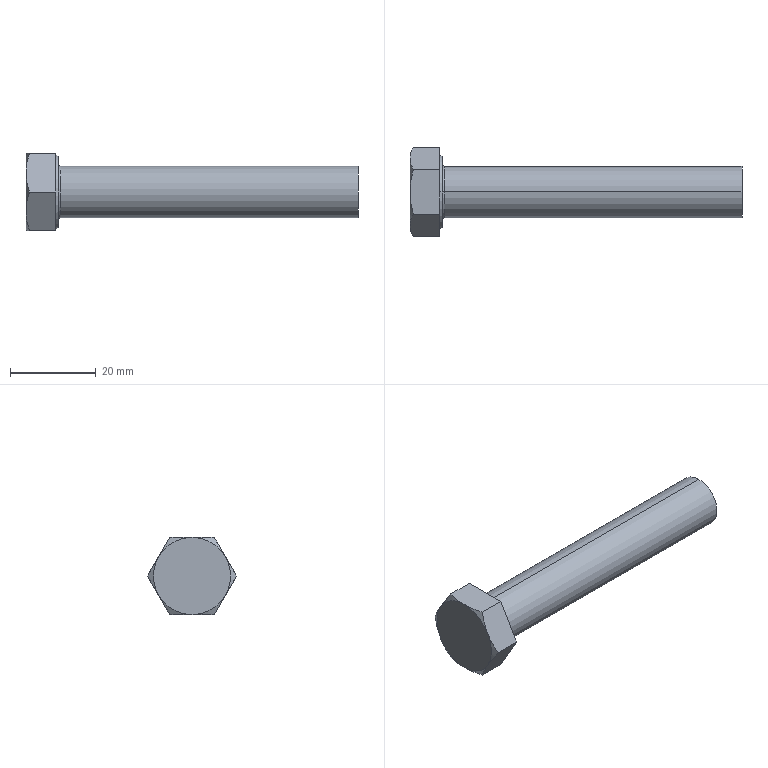Part | SolidWorks | features RevCut 3, Extrusion 1, Fillet 1, LPattern 1, Revolution 1 | 1 solid | 22 faces | box 77.5 x 20.785 x 18 mm | volume 9985 mm3 | plane 10 | cone 8 | torus 2 | cylinder 2 | commonest cylinder face diameters 12 x2
STEP:
#1=CARTESIAN_POINT('',(8.1,0.,6.));
#2=VERTEX_POINT('',#1);
#3=CARTESIAN_POINT('',(8.1,0.,-6.));
#4=VERTEX_POINT('',#3);
#5=CARTESIAN_POINT('',(8.1,0.,0.));
#6=DIRECTION('',(1.,0.,0.));
#7=DIRECTION('',(0.,0.,-1.));
#8=AXIS2_PLACEMENT_3D('',#5,#6,#7);
#9=CIRCLE('',#8,6.);
#10=EDGE_CURVE('',#2,#4,#9,.T.);
#11=ORIENTED_EDGE('',*,*,#10,.F.);
#12=CARTESIAN_POINT('',(7.5,0.,6.6));
#13=VERTEX_POINT('',#12);
#14=CARTESIAN_POINT('',(8.1,0.,6.6));
#15=DIRECTION('',(0.,1.,0.));
#16=DIRECTION('',(0.,0.,1.));
#17=AXIS2_PLACEMENT_3D('',#14,#15,#16);
#18=CIRCLE('',#17,0.6);
#19=EDGE_CURVE('',#2,#13,#18,.T.);
#20=ORIENTED_EDGE('',*,*,#19,.T.);
#21=CARTESIAN_POINT('',(7.5,0.,-6.6));
#22=VERTEX_POINT('',#21);
#23=CARTESIAN_POINT('',(7.5,0.,0.));
#24=DIRECTION('',(-1.,0.,0.));
#25=DIRECTION('',(0.,0.,-1.));
#26=AXIS2_PLACEMENT_3D('',#23,#24,#25);
#27=CIRCLE('',#26,6.6);
#28=EDGE_CURVE('',#22,#13,#27,.T.);
#29=ORIENTED_EDGE('',*,*,#28,.F.);
#30=CARTESIAN_POINT('',(8.1,0.,-6.6));
#31=DIRECTION('',(0.,-1.,0.));
#32=DIRECTION('',(0.,0.,-1.));
#33=AXIS2_PLACEMENT_3D('',#30,#31,#32);
#34=CIRCLE('',#33,0.6);
#35=EDGE_CURVE('',#4,#22,#34,.T.);
#36=ORIENTED_EDGE('',*,*,#35,.F.);
#37=EDGE_LOOP('',(#11,#20,#29,#36));
#38=FACE_OUTER_BOUND('',#37,.T.);
#39=CARTESIAN_POINT('',(8.1,0.,0.));
#40=DIRECTION('',(1.,0.,0.));
#41=DIRECTION('',(0.,0.,-1.));
#42=AXIS2_PLACEMENT_3D('',#39,#40,#41);
#43=TOROIDAL_SURFACE('',#42,6.6,0.6);
#44=ADVANCED_FACE('',(#38),#43,.F.);
#45=CARTESIAN_POINT('',(77.5,0.,6.));
#46=VERTEX_POINT('',#45);
#47=CARTESIAN_POINT('',(77.5,0.,-6.));
#48=VERTEX_POINT('',#47);
#49=CARTESIAN_POINT('',(77.5,0.,0.));
#50=DIRECTION('',(-1.,0.,0.));
#51=DIRECTION('',(0.,0.,1.));
#52=AXIS2_PLACEMENT_3D('',#49,#50,#51);
#53=CIRCLE('',#52,6.);
#54=EDGE_CURVE('',#46,#48,#53,.T.);
#55=ORIENTED_EDGE('',*,*,#54,.T.);
#56=CARTESIAN_POINT('',(0.,0.,-6.));
#57=DIRECTION('',(-1.,0.,0.));
#58=VECTOR('',#57,1000.);
#59=LINE('',#56,#58);
#60=EDGE_CURVE('',#48,#4,#59,.T.);
#61=ORIENTED_EDGE('',*,*,#60,.T.);
#62=CARTESIAN_POINT('',(8.1,0.,0.));
#63=DIRECTION('',(1.,0.,0.));
#64=DIRECTION('',(0.,0.,-1.));
#65=AXIS2_PLACEMENT_3D('',#62,#63,#64);
#66=CIRCLE('',#65,6.);
#67=EDGE_CURVE('',#4,#2,#66,.T.);
#68=ORIENTED_EDGE('',*,*,#67,.T.);
#69=CARTESIAN_POINT('',(0.,0.,6.));
#70=DIRECTION('',(-1.,0.,0.));
#71=VECTOR('',#70,1000.);
#72=LINE('',#69,#71);
#73=EDGE_CURVE('',#46,#2,#72,.T.);
#74=ORIENTED_EDGE('',*,*,#73,.F.);
#75=EDGE_LOOP('',(#55,#61,#68,#74));
#76=FACE_OUTER_BOUND('',#75,.T.);
#77=CARTESIAN_POINT('',(0.,0.,0.));
#78=DIRECTION('',(-1.,0.,0.));
#79=DIRECTION('',(0.,0.,1.));
#80=AXIS2_PLACEMENT_3D('',#77,#78,#79);
#81=CYLINDRICAL_SURFACE('',#80,6.);
#82=ADVANCED_FACE('',(#76),#81,.T.);
#83=CARTESIAN_POINT('',(7.5,0.,8.315));
#84=VERTEX_POINT('',#83);
#85=CARTESIAN_POINT('',(7.5,0.,-8.315));
#86=VERTEX_POINT('',#85);
#87=CARTESIAN_POINT('',(7.5,0.,0.));
#88=DIRECTION('',(-1.,0.,0.));
#89=DIRECTION('',(0.,0.,1.));
#90=AXIS2_PLACEMENT_3D('',#87,#88,#89);
#91=CIRCLE('',#90,8.315);
#92=EDGE_CURVE('',#84,#86,#91,.T.);
#93=ORIENTED_EDGE('',*,*,#92,.T.);
#94=CARTESIAN_POINT('',(6.9,0.,-8.661));
#95=VERTEX_POINT('',#94);
#96=CARTESIAN_POINT('',(6.9,0.,-8.661));
#97=DIRECTION('',(-0.866,0.,-0.5));
#98=VECTOR('',#97,1000.);
#99=LINE('',#96,#98);
#100=EDGE_CURVE('',#86,#95,#99,.T.);
#101=ORIENTED_EDGE('',*,*,#100,.T.);
#102=CARTESIAN_POINT('',(6.9,0.,8.661));
#103=VERTEX_POINT('',#102);
#104=CARTESIAN_POINT('',(6.9,0.,0.));
#105=DIRECTION('',(-1.,0.,0.));
#106=DIRECTION('',(0.,0.,1.));
#107=AXIS2_PLACEMENT_3D('',#104,#105,#106);
#108=CIRCLE('',#107,8.661);
#109=EDGE_CURVE('',#103,#95,#108,.T.);
#110=ORIENTED_EDGE('',*,*,#109,.F.);
#111=CARTESIAN_POINT('',(6.9,0.,8.661));
#112=DIRECTION('',(-0.866,0.,0.5));
#113=VECTOR('',#112,1000.);
#114=LINE('',#111,#113);
#115=EDGE_CURVE('',#84,#103,#114,.T.);
#116=ORIENTED_EDGE('',*,*,#115,.F.);
#117=EDGE_LOOP('',(#93,#101,#110,#116));
#118=FACE_OUTER_BOUND('',#117,.T.);
#119=CARTESIAN_POINT('',(6.9,0.,0.));
#120=DIRECTION('',(-1.,0.,0.));
#121=DIRECTION('',(0.,0.,1.));
#122=AXIS2_PLACEMENT_3D('',#119,#120,#121);
#123=CONICAL_SURFACE('',#122,8.661,0.5236);
#124=ADVANCED_FACE('',(#118),#123,.T.);
#125=CARTESIAN_POINT('',(6.9,5.196,-9.));
#126=VERTEX_POINT('',#125);
#127=CARTESIAN_POINT('',(6.9,10.392,0.));
#128=VERTEX_POINT('',#127);
#129=CARTESIAN_POINT('',(6.9,5.196,-9.));
#130=DIRECTION('',(0.,0.5,0.866));
#131=VECTOR('',#130,1000.);
#132=LINE('',#129,#131);
#133=EDGE_CURVE('',#126,#128,#132,.T.);
#134=ORIENTED_EDGE('',*,*,#133,.F.);
#135=CARTESIAN_POINT('',(0.8038,5.196,-9.));
#136=VERTEX_POINT('',#135);
#137=CARTESIAN_POINT('',(7.5,5.196,-9.));
#138=DIRECTION('',(-1.,0.,0.));
#139=VECTOR('',#138,1000.);
#140=LINE('',#137,#139);
#141=EDGE_CURVE('',#126,#136,#140,.T.);
#142=ORIENTED_EDGE('',*,*,#141,.T.);
#143=CARTESIAN_POINT('',(0.,7.794,-4.5));
#144=VERTEX_POINT('',#143);
#145=CARTESIAN_POINT('',(0.,7.794,-4.5));
#146=CARTESIAN_POINT('',(0.,7.574,-4.882));
#147=CARTESIAN_POINT('',(0.019,7.352,-5.266));
#148=CARTESIAN_POINT('',(0.09253,6.914,-6.024));
#149=CARTESIAN_POINT('',(0.147,6.697,-6.401));
#150=CARTESIAN_POINT('',(0.357,6.048,-7.525));
#151=CARTESIAN_POINT('',(0.5591,5.62,-8.266));
#152=CARTESIAN_POINT('',(0.8038,5.196,-9.));
#153=B_SPLINE_CURVE_WITH_KNOTS('',3,(#145,#146,#147,#148,#149,#150,#151,#152),.UNSPECIFIED.,.F.,.F.,(4,2,2,4),(0.005258,0.006567,0.007877,0.0105),.UNSPECIFIED.);
#154=EDGE_CURVE('',#144,#136,#153,.T.);
#155=ORIENTED_EDGE('',*,*,#154,.F.);
#156=CARTESIAN_POINT('',(0.8038,10.392,0.));
#157=VERTEX_POINT('',#156);
#158=CARTESIAN_POINT('',(0.8038,10.392,0.));
#159=CARTESIAN_POINT('',(0.5585,9.967,-0.7361));
#160=CARTESIAN_POINT('',(0.3563,9.539,-1.478));
#161=CARTESIAN_POINT('',(0.07661,8.674,-2.976));
#162=CARTESIAN_POINT('',(0.,8.237,-3.733));
#163=CARTESIAN_POINT('',(0.,7.794,-4.5));
#164=B_SPLINE_CURVE_WITH_KNOTS('',3,(#158,#159,#160,#161,#162,#163),.UNSPECIFIED.,.F.,.F.,(4,2,4),(0.000000238,0.002629,0.005258),.UNSPECIFIED.);
#165=EDGE_CURVE('',#157,#144,#164,.T.);
#166=ORIENTED_EDGE('',*,*,#165,.F.);
#167=CARTESIAN_POINT('',(7.5,10.392,0.));
#168=DIRECTION('',(-1.,0.,0.));
#169=VECTOR('',#168,1000.);
#170=LINE('',#167,#169);
#171=EDGE_CURVE('',#128,#157,#170,.T.);
#172=ORIENTED_EDGE('',*,*,#171,.F.);
#173=EDGE_LOOP('',(#134,#142,#155,#166,#172));
#174=FACE_OUTER_BOUND('',#173,.T.);
#175=CARTESIAN_POINT('',(7.5,5.196,-9.));
#176=DIRECTION('',(0.,-0.866,0.5));
#177=DIRECTION('',(0.,-0.5,-0.866));
#178=AXIS2_PLACEMENT_3D('',#175,#176,#177);
#179=PLANE('',#178);
#180=ADVANCED_FACE('',(#174),#179,.F.);
#181=CARTESIAN_POINT('',(6.9,5.196,9.));
#182=VERTEX_POINT('',#181);
#183=CARTESIAN_POINT('',(6.9,10.392,0.));
#184=DIRECTION('',(0.,-0.5,0.866));
#185=VECTOR('',#184,1000.);
#186=LINE('',#183,#185);
#187=EDGE_CURVE('',#128,#182,#186,.T.);
#188=ORIENTED_EDGE('',*,*,#187,.F.);
#189=ORIENTED_EDGE('',*,*,#171,.T.);
#190=CARTESIAN_POINT('',(0.,7.794,4.5));
#191=VERTEX_POINT('',#190);
#192=CARTESIAN_POINT('',(0.,7.794,4.5));
#193=CARTESIAN_POINT('',(0.,8.015,4.118));
#194=CARTESIAN_POINT('',(0.019,8.236,3.734));
#195=CARTESIAN_POINT('',(0.09253,8.674,2.976));
#196=CARTESIAN_POINT('',(0.147,8.892,2.599));
#197=CARTESIAN_POINT('',(0.357,9.541,1.475));
#198=CARTESIAN_POINT('',(0.5591,9.968,0.7343));
#199=CARTESIAN_POINT('',(0.8038,10.392,0.));
#200=B_SPLINE_CURVE_WITH_KNOTS('',3,(#192,#193,#194,#195,#196,#197,#198,#199),.UNSPECIFIED.,.F.,.F.,(4,2,2,4),(0.005258,0.006567,0.007877,0.0105),.UNSPECIFIED.);
#201=EDGE_CURVE('',#191,#157,#200,.T.);
#202=ORIENTED_EDGE('',*,*,#201,.F.);
#203=CARTESIAN_POINT('',(0.8038,5.196,9.));
#204=VERTEX_POINT('',#203);
#205=CARTESIAN_POINT('',(0.8038,5.196,9.));
#206=CARTESIAN_POINT('',(0.5585,5.621,8.264));
#207=CARTESIAN_POINT('',(0.3563,6.049,7.522));
#208=CARTESIAN_POINT('',(0.07661,6.914,6.024));
#209=CARTESIAN_POINT('',(0.,7.352,5.267));
#210=CARTESIAN_POINT('',(0.,7.794,4.5));
#211=B_SPLINE_CURVE_WITH_KNOTS('',3,(#205,#206,#207,#208,#209,#210),.UNSPECIFIED.,.F.,.F.,(4,2,4),(0.000000238,0.002629,0.005258),.UNSPECIFIED.);
#212=EDGE_CURVE('',#204,#191,#211,.T.);
#213=ORIENTED_EDGE('',*,*,#212,.F.);
#214=CARTESIAN_POINT('',(7.5,5.196,9.));
#215=DIRECTION('',(-1.,0.,0.));
#216=VECTOR('',#215,1000.);
#217=LINE('',#214,#216);
#218=EDGE_CURVE('',#182,#204,#217,.T.);
#219=ORIENTED_EDGE('',*,*,#218,.F.);
#220=EDGE_LOOP('',(#188,#189,#202,#213,#219));
#221=FACE_OUTER_BOUND('',#220,.T.);
#222=CARTESIAN_POINT('',(7.5,10.392,0.));
#223=DIRECTION('',(0.,-0.866,-0.5));
#224=DIRECTION('',(0.,0.5,-0.866));
#225=AXIS2_PLACEMENT_3D('',#222,#223,#224);
#226=PLANE('',#225);
#227=ADVANCED_FACE('',(#221),#226,.F.);
#228=CARTESIAN_POINT('',(6.9,-5.196,9.));
#229=VERTEX_POINT('',#228);
#230=CARTESIAN_POINT('',(6.9,5.196,9.));
#231=DIRECTION('',(0.,-1.,0.));
#232=VECTOR('',#231,1000.);
#233=LINE('',#230,#232);
#234=EDGE_CURVE('',#182,#229,#233,.T.);
#235=ORIENTED_EDGE('',*,*,#234,.F.);
#236=ORIENTED_EDGE('',*,*,#218,.T.);
#237=CARTESIAN_POINT('',(0.,0.,9.));
#238=VERTEX_POINT('',#237);
#239=CARTESIAN_POINT('',(0.,0.,9.));
#240=CARTESIAN_POINT('',(0.,0.4401,9.));
#241=CARTESIAN_POINT('',(0.01885,0.8832,9.));
#242=CARTESIAN_POINT('',(0.09319,1.767,9.));
#243=CARTESIAN_POINT('',(0.1482,2.204,9.));
#244=CARTESIAN_POINT('',(0.3593,3.505,9.));
#245=CARTESIAN_POINT('',(0.5612,4.356,9.));
#246=CARTESIAN_POINT('',(0.8038,5.196,9.));
#247=B_SPLINE_CURVE_WITH_KNOTS('',3,(#239,#240,#241,#242,#243,#244,#245,#246),.UNSPECIFIED.,.F.,.F.,(4,2,2,4),(0.01498,0.0163,0.01761,0.02025),.UNSPECIFIED.);
#248=EDGE_CURVE('',#238,#204,#247,.T.);
#249=ORIENTED_EDGE('',*,*,#248,.F.);
#250=CARTESIAN_POINT('',(0.8038,-5.196,9.));
#251=VERTEX_POINT('',#250);
#252=CARTESIAN_POINT('',(0.8038,-5.196,9.));
#253=CARTESIAN_POINT('',(0.5595,-4.35,9.));
#254=CARTESIAN_POINT('',(0.3552,-3.485,9.));
#255=CARTESIAN_POINT('',(0.07569,-1.752,9.));
#256=CARTESIAN_POINT('',(0.,-0.8794,9.));
#257=CARTESIAN_POINT('',(0.,0.,9.));
#258=B_SPLINE_CURVE_WITH_KNOTS('',3,(#252,#253,#254,#255,#256,#257),.UNSPECIFIED.,.F.,.F.,(4,2,4),(0.00972,0.01235,0.01498),.UNSPECIFIED.);
#259=EDGE_CURVE('',#251,#238,#258,.T.);
#260=ORIENTED_EDGE('',*,*,#259,.F.);
#261=CARTESIAN_POINT('',(7.5,-5.196,9.));
#262=DIRECTION('',(-1.,0.,0.));
#263=VECTOR('',#262,1000.);
#264=LINE('',#261,#263);
#265=EDGE_CURVE('',#229,#251,#264,.T.);
#266=ORIENTED_EDGE('',*,*,#265,.F.);
#267=EDGE_LOOP('',(#235,#236,#249,#260,#266));
#268=FACE_OUTER_BOUND('',#267,.T.);
#269=CARTESIAN_POINT('',(7.5,5.196,9.));
#270=DIRECTION('',(0.,0.,-1.));
#271=DIRECTION('',(-1.,0.,0.));
#272=AXIS2_PLACEMENT_3D('',#269,#270,#271);
#273=PLANE('',#272);
#274=ADVANCED_FACE('',(#268),#273,.F.);
#275=CARTESIAN_POINT('',(6.9,-10.392,0.));
#276=VERTEX_POINT('',#275);
#277=CARTESIAN_POINT('',(6.9,-10.392,0.));
#278=DIRECTION('',(0.,-0.5,-0.866));
#279=VECTOR('',#278,1000.);
#280=LINE('',#277,#279);
#281=EDGE_CURVE('',#229,#276,#280,.T.);
#282=ORIENTED_EDGE('',*,*,#281,.F.);
#283=ORIENTED_EDGE('',*,*,#265,.T.);
#284=CARTESIAN_POINT('',(0.,-7.794,4.5));
#285=VERTEX_POINT('',#284);
#286=CARTESIAN_POINT('',(0.,-7.794,4.5));
#287=CARTESIAN_POINT('',(0.,-7.574,4.882));
#288=CARTESIAN_POINT('',(0.019,-7.352,5.266));
#289=CARTESIAN_POINT('',(0.09253,-6.914,6.024));
#290=CARTESIAN_POINT('',(0.147,-6.697,6.401));
#291=CARTESIAN_POINT('',(0.357,-6.048,7.525));
#292=CARTESIAN_POINT('',(0.5591,-5.62,8.266));
#293=CARTESIAN_POINT('',(0.8038,-5.196,9.));
#294=B_SPLINE_CURVE_WITH_KNOTS('',3,(#286,#287,#288,#289,#290,#291,#292,#293),.UNSPECIFIED.,.F.,.F.,(4,2,2,4),(0.005258,0.006567,0.007877,0.0105),.UNSPECIFIED.);
#295=EDGE_CURVE('',#285,#251,#294,.T.);
#296=ORIENTED_EDGE('',*,*,#295,.F.);
#297=CARTESIAN_POINT('',(0.8038,-10.392,0.));
#298=VERTEX_POINT('',#297);
#299=CARTESIAN_POINT('',(0.8038,-10.392,0.));
#300=CARTESIAN_POINT('',(0.5585,-9.967,0.7361));
#301=CARTESIAN_POINT('',(0.3563,-9.539,1.478));
#302=CARTESIAN_POINT('',(0.07661,-8.674,2.976));
#303=CARTESIAN_POINT('',(0.,-8.237,3.733));
#304=CARTESIAN_POINT('',(0.,-7.794,4.5));
#305=B_SPLINE_CURVE_WITH_KNOTS('',3,(#299,#300,#301,#302,#303,#304),.UNSPECIFIED.,.F.,.F.,(4,2,4),(0.000000238,0.002629,0.005258),.UNSPECIFIED.);
#306=EDGE_CURVE('',#298,#285,#305,.T.);
#307=ORIENTED_EDGE('',*,*,#306,.F.);
#308=CARTESIAN_POINT('',(7.5,-10.392,0.));
#309=DIRECTION('',(-1.,0.,0.));
#310=VECTOR('',#309,1000.);
#311=LINE('',#308,#310);
#312=EDGE_CURVE('',#276,#298,#311,.T.);
#313=ORIENTED_EDGE('',*,*,#312,.F.);
#314=EDGE_LOOP('',(#282,#283,#296,#307,#313));
#315=FACE_OUTER_BOUND('',#314,.T.);
#316=CARTESIAN_POINT('',(7.5,-10.392,0.));
#317=DIRECTION('',(0.,0.866,-0.5));
#318=DIRECTION('',(0.,0.5,0.866));
#319=AXIS2_PLACEMENT_3D('',#316,#317,#318);
#320=PLANE('',#319);
#321=ADVANCED_FACE('',(#315),#320,.F.);
#322=CARTESIAN_POINT('',(6.9,-5.196,-9.));
#323=VERTEX_POINT('',#322);
#324=CARTESIAN_POINT('',(6.9,-5.196,-9.));
#325=DIRECTION('',(0.,0.5,-0.866));
#326=VECTOR('',#325,1000.);
#327=LINE('',#324,#326);
#328=EDGE_CURVE('',#276,#323,#327,.T.);
#329=ORIENTED_EDGE('',*,*,#328,.F.);
#330=ORIENTED_EDGE('',*,*,#312,.T.);
#331=CARTESIAN_POINT('',(0.,-7.794,-4.5));
#332=VERTEX_POINT('',#331);
#333=CARTESIAN_POINT('',(0.,-7.794,-4.5));
#334=CARTESIAN_POINT('',(0.,-8.015,-4.118));
#335=CARTESIAN_POINT('',(0.019,-8.236,-3.734));
#336=CARTESIAN_POINT('',(0.09253,-8.674,-2.976));
#337=CARTESIAN_POINT('',(0.147,-8.892,-2.599));
#338=CARTESIAN_POINT('',(0.357,-9.541,-1.475));
#339=CARTESIAN_POINT('',(0.5591,-9.968,-0.7343));
#340=CARTESIAN_POINT('',(0.8038,-10.392,0.));
#341=B_SPLINE_CURVE_WITH_KNOTS('',3,(#333,#334,#335,#336,#337,#338,#339,#340),.UNSPECIFIED.,.F.,.F.,(4,2,2,4),(0.005258,0.006567,0.007877,0.0105),.UNSPECIFIED.);
#342=EDGE_CURVE('',#332,#298,#341,.T.);
#343=ORIENTED_EDGE('',*,*,#342,.F.);
#344=CARTESIAN_POINT('',(0.8038,-5.196,-9.));
#345=VERTEX_POINT('',#344);
#346=CARTESIAN_POINT('',(0.8038,-5.196,-9.));
#347=CARTESIAN_POINT('',(0.5585,-5.621,-8.264));
#348=CARTESIAN_POINT('',(0.3563,-6.049,-7.522));
#349=CARTESIAN_POINT('',(0.07661,-6.914,-6.024));
#350=CARTESIAN_POINT('',(0.,-7.352,-5.267));
#351=CARTESIAN_POINT('',(0.,-7.794,-4.5));
#352=B_SPLINE_CURVE_WITH_KNOTS('',3,(#346,#347,#348,#349,#350,#351),.UNSPECIFIED.,.F.,.F.,(4,2,4),(0.000000238,0.002629,0.005258),.UNSPECIFIED.);
#353=EDGE_CURVE('',#345,#332,#352,.T.);
#354=ORIENTED_EDGE('',*,*,#353,.F.);
#355=CARTESIAN_POINT('',(7.5,-5.196,-9.));
#356=DIRECTION('',(-1.,0.,0.));
#357=VECTOR('',#356,1000.);
#358=LINE('',#355,#357);
#359=EDGE_CURVE('',#323,#345,#358,.T.);
#360=ORIENTED_EDGE('',*,*,#359,.F.);
#361=EDGE_LOOP('',(#329,#330,#343,#354,#360));
#362=FACE_OUTER_BOUND('',#361,.T.);
#363=CARTESIAN_POINT('',(7.5,-5.196,-9.));
#364=DIRECTION('',(0.,0.866,0.5));
#365=DIRECTION('',(0.,-0.5,0.866));
#366=AXIS2_PLACEMENT_3D('',#363,#364,#365);
#367=PLANE('',#366);
#368=ADVANCED_FACE('',(#362),#367,.F.);
#369=CARTESIAN_POINT('',(6.9,5.196,-9.));
#370=DIRECTION('',(0.,1.,0.));
#371=VECTOR('',#370,1000.);
#372=LINE('',#369,#371);
#373=EDGE_CURVE('',#323,#126,#372,.T.);
#374=ORIENTED_EDGE('',*,*,#373,.F.);
#375=ORIENTED_EDGE('',*,*,#359,.T.);
#376=CARTESIAN_POINT('',(0.,0.,-9.));
#377=VERTEX_POINT('',#376);
#378=CARTESIAN_POINT('',(0.,0.,-9.));
#379=CARTESIAN_POINT('',(0.,-0.8794,-9.));
#380=CARTESIAN_POINT('',(0.07569,-1.752,-9.));
#381=CARTESIAN_POINT('',(0.3552,-3.485,-9.));
#382=CARTESIAN_POINT('',(0.5595,-4.35,-9.));
#383=CARTESIAN_POINT('',(0.8038,-5.196,-9.));
#384=B_SPLINE_CURVE_WITH_KNOTS('',3,(#378,#379,#380,#381,#382,#383),.UNSPECIFIED.,.F.,.F.,(4,2,4),(0.03045,0.03308,0.03571),.UNSPECIFIED.);
#385=EDGE_CURVE('',#377,#345,#384,.T.);
#386=ORIENTED_EDGE('',*,*,#385,.F.);
#387=CARTESIAN_POINT('',(0.8038,5.196,-9.));
#388=CARTESIAN_POINT('',(0.5612,4.356,-9.));
#389=CARTESIAN_POINT('',(0.3593,3.505,-9.));
#390=CARTESIAN_POINT('',(0.1482,2.204,-9.));
#391=CARTESIAN_POINT('',(0.09319,1.767,-9.));
#392=CARTESIAN_POINT('',(0.01885,0.8832,-9.));
#393=CARTESIAN_POINT('',(0.,0.4401,-9.));
#394=CARTESIAN_POINT('',(0.,0.,-9.));
#395=B_SPLINE_CURVE_WITH_KNOTS('',3,(#387,#388,#389,#390,#391,#392,#393,#394),.UNSPECIFIED.,.F.,.F.,(4,2,2,4),(0.02519,0.02782,0.02914,0.03045),.UNSPECIFIED.);
#396=EDGE_CURVE('',#136,#377,#395,.T.);
#397=ORIENTED_EDGE('',*,*,#396,.F.);
#398=ORIENTED_EDGE('',*,*,#141,.F.);
#399=EDGE_LOOP('',(#374,#375,#386,#397,#398));
#400=FACE_OUTER_BOUND('',#399,.T.);
#401=CARTESIAN_POINT('',(7.5,5.196,-9.));
#402=DIRECTION('',(0.,0.,1.));
#403=DIRECTION('',(0.,-1.,0.));
#404=AXIS2_PLACEMENT_3D('',#401,#402,#403);
#405=PLANE('',#404);
#406=ADVANCED_FACE('',(#400),#405,.F.);
#407=ORIENTED_EDGE('',*,*,#353,.T.);
#408=CARTESIAN_POINT('',(0.,0.,0.));
#409=DIRECTION('',(1.,0.,0.));
#410=DIRECTION('',(0.,0.,-1.));
#411=AXIS2_PLACEMENT_3D('',#408,#409,#410);
#412=CIRCLE('',#411,9.);
#413=EDGE_CURVE('',#332,#377,#412,.T.);
#414=ORIENTED_EDGE('',*,*,#413,.T.);
#415=ORIENTED_EDGE('',*,*,#385,.T.);
#416=EDGE_LOOP('',(#407,#414,#415));
#417=FACE_OUTER_BOUND('',#416,.T.);
#418=CARTESIAN_POINT('',(0.,0.,0.));
#419=DIRECTION('',(1.,0.,0.));
#420=DIRECTION('',(0.,0.,-1.));
#421=AXIS2_PLACEMENT_3D('',#418,#419,#420);
#422=CONICAL_SURFACE('',#421,9.,1.047);
#423=ADVANCED_FACE('',(#417),#422,.T.);
#424=ORIENTED_EDGE('',*,*,#306,.T.);
#425=CARTESIAN_POINT('',(0.,0.,0.));
#426=DIRECTION('',(1.,0.,0.));
#427=DIRECTION('',(0.,0.,-1.));
#428=AXIS2_PLACEMENT_3D('',#425,#426,#427);
#429=CIRCLE('',#428,9.);
#430=EDGE_CURVE('',#285,#332,#429,.T.);
#431=ORIENTED_EDGE('',*,*,#430,.T.);
#432=ORIENTED_EDGE('',*,*,#342,.T.);
#433=EDGE_LOOP('',(#424,#431,#432));
#434=FACE_OUTER_BOUND('',#433,.T.);
#435=CARTESIAN_POINT('',(0.,0.,0.));
#436=DIRECTION('',(1.,0.,0.));
#437=DIRECTION('',(0.,0.,-1.));
#438=AXIS2_PLACEMENT_3D('',#435,#436,#437);
#439=CONICAL_SURFACE('',#438,9.,1.047);
#440=ADVANCED_FACE('',(#434),#439,.T.);
#441=ORIENTED_EDGE('',*,*,#259,.T.);
#442=CARTESIAN_POINT('',(0.,0.,0.));
#443=DIRECTION('',(1.,0.,0.));
#444=DIRECTION('',(0.,0.,-1.));
#445=AXIS2_PLACEMENT_3D('',#442,#443,#444);
#446=CIRCLE('',#445,9.);
#447=EDGE_CURVE('',#238,#285,#446,.T.);
#448=ORIENTED_EDGE('',*,*,#447,.T.);
#449=ORIENTED_EDGE('',*,*,#295,.T.);
#450=EDGE_LOOP('',(#441,#448,#449));
#451=FACE_OUTER_BOUND('',#450,.T.);
#452=CARTESIAN_POINT('',(0.,0.,0.));
#453=DIRECTION('',(1.,0.,0.));
#454=DIRECTION('',(0.,0.,-1.));
#455=AXIS2_PLACEMENT_3D('',#452,#453,#454);
#456=CONICAL_SURFACE('',#455,9.,1.047);
#457=ADVANCED_FACE('',(#451),#456,.T.);
#458=ORIENTED_EDGE('',*,*,#248,.T.);
#459=ORIENTED_EDGE('',*,*,#212,.T.);
#460=CARTESIAN_POINT('',(0.,0.,0.));
#461=DIRECTION('',(-1.,0.,0.));
#462=DIRECTION('',(0.,0.,1.));
#463=AXIS2_PLACEMENT_3D('',#460,#461,#462);
#464=CIRCLE('',#463,9.);
#465=EDGE_CURVE('',#238,#191,#464,.T.);
#466=ORIENTED_EDGE('',*,*,#465,.F.);
#467=EDGE_LOOP('',(#458,#459,#466));
#468=FACE_OUTER_BOUND('',#467,.T.);
#469=CARTESIAN_POINT('',(0.,0.,0.));
#470=DIRECTION('',(1.,0.,0.));
#471=DIRECTION('',(0.,0.,-1.));
#472=AXIS2_PLACEMENT_3D('',#469,#470,#471);
#473=CONICAL_SURFACE('',#472,9.,1.047);
#474=ADVANCED_FACE('',(#468),#473,.T.);
#475=ORIENTED_EDGE('',*,*,#201,.T.);
#476=ORIENTED_EDGE('',*,*,#165,.T.);
#477=CARTESIAN_POINT('',(0.,0.,0.));
#478=DIRECTION('',(1.,0.,0.));
#479=DIRECTION('',(0.,0.,-1.));
#480=AXIS2_PLACEMENT_3D('',#477,#478,#479);
#481=CIRCLE('',#480,9.);
#482=EDGE_CURVE('',#144,#191,#481,.T.);
#483=ORIENTED_EDGE('',*,*,#482,.T.);
#484=EDGE_LOOP('',(#475,#476,#483));
#485=FACE_OUTER_BOUND('',#484,.T.);
#486=CARTESIAN_POINT('',(0.,0.,0.));
#487=DIRECTION('',(1.,0.,0.));
#488=DIRECTION('',(0.,0.,-1.));
#489=AXIS2_PLACEMENT_3D('',#486,#487,#488);
#490=CONICAL_SURFACE('',#489,9.,1.047);
#491=ADVANCED_FACE('',(#485),#490,.T.);
#492=ORIENTED_EDGE('',*,*,#154,.T.);
#493=ORIENTED_EDGE('',*,*,#396,.T.);
#494=CARTESIAN_POINT('',(0.,0.,0.));
#495=DIRECTION('',(1.,0.,0.));
#496=DIRECTION('',(0.,0.,-1.));
#497=AXIS2_PLACEMENT_3D('',#494,#495,#496);
#498=CIRCLE('',#497,9.);
#499=EDGE_CURVE('',#377,#144,#498,.T.);
#500=ORIENTED_EDGE('',*,*,#499,.T.);
#501=EDGE_LOOP('',(#492,#493,#500));
#502=FACE_OUTER_BOUND('',#501,.T.);
#503=CARTESIAN_POINT('',(0.,0.,0.));
#504=DIRECTION('',(1.,0.,0.));
#505=DIRECTION('',(0.,0.,-1.));
#506=AXIS2_PLACEMENT_3D('',#503,#504,#505);
#507=CONICAL_SURFACE('',#506,9.,1.047);
#508=ADVANCED_FACE('',(#502),#507,.T.);
#509=ORIENTED_EDGE('',*,*,#499,.F.);
#510=ORIENTED_EDGE('',*,*,#413,.F.);
#511=ORIENTED_EDGE('',*,*,#430,.F.);
#512=ORIENTED_EDGE('',*,*,#447,.F.);
#513=ORIENTED_EDGE('',*,*,#465,.T.);
#514=ORIENTED_EDGE('',*,*,#482,.F.);
#515=EDGE_LOOP('',(#509,#510,#511,#512,#513,#514));
#516=FACE_OUTER_BOUND('',#515,.T.);
#517=CARTESIAN_POINT('',(0.,10.392,0.));
#518=DIRECTION('',(1.,0.,0.));
#519=DIRECTION('',(0.,0.,-1.));
#520=AXIS2_PLACEMENT_3D('',#517,#518,#519);
#521=PLANE('',#520);
#522=ADVANCED_FACE('',(#516),#521,.F.);
#523=ORIENTED_EDGE('',*,*,#109,.T.);
#524=CARTESIAN_POINT('',(6.9,0.,0.));
#525=DIRECTION('',(-1.,0.,0.));
#526=DIRECTION('',(0.,0.,1.));
#527=AXIS2_PLACEMENT_3D('',#524,#525,#526);
#528=CIRCLE('',#527,8.661);
#529=EDGE_CURVE('',#95,#103,#528,.T.);
#530=ORIENTED_EDGE('',*,*,#529,.T.);
#531=EDGE_LOOP('',(#523,#530));
#532=FACE_BOUND('',#531,.T.);
#533=ORIENTED_EDGE('',*,*,#133,.T.);
#534=ORIENTED_EDGE('',*,*,#187,.T.);
#535=ORIENTED_EDGE('',*,*,#234,.T.);
#536=ORIENTED_EDGE('',*,*,#281,.T.);
#537=ORIENTED_EDGE('',*,*,#328,.T.);
#538=ORIENTED_EDGE('',*,*,#373,.T.);
#539=EDGE_LOOP('',(#533,#534,#535,#536,#537,#538));
#540=FACE_OUTER_BOUND('',#539,.T.);
#541=CARTESIAN_POINT('',(6.9,8.661,0.));
#542=DIRECTION('',(1.,0.,0.));
#543=DIRECTION('',(0.,0.,-1.));
#544=AXIS2_PLACEMENT_3D('',#541,#542,#543);
#545=PLANE('',#544);
#546=ADVANCED_FACE('',(#532,#540),#545,.T.);
#547=ORIENTED_EDGE('',*,*,#100,.F.);
#548=CARTESIAN_POINT('',(7.5,0.,0.));
#549=DIRECTION('',(-1.,0.,0.));
#550=DIRECTION('',(0.,0.,1.));
#551=AXIS2_PLACEMENT_3D('',#548,#549,#550);
#552=CIRCLE('',#551,8.315);
#553=EDGE_CURVE('',#86,#84,#552,.T.);
#554=ORIENTED_EDGE('',*,*,#553,.T.);
#555=ORIENTED_EDGE('',*,*,#115,.T.);
#556=ORIENTED_EDGE('',*,*,#529,.F.);
#557=EDGE_LOOP('',(#547,#554,#555,#556));
#558=FACE_OUTER_BOUND('',#557,.T.);
#559=CARTESIAN_POINT('',(6.9,0.,0.));
#560=DIRECTION('',(-1.,0.,0.));
#561=DIRECTION('',(0.,0.,1.));
#562=AXIS2_PLACEMENT_3D('',#559,#560,#561);
#563=CONICAL_SURFACE('',#562,8.661,0.5236);
#564=ADVANCED_FACE('',(#558),#563,.T.);
#565=ORIENTED_EDGE('',*,*,#54,.F.);
#566=CARTESIAN_POINT('',(77.5,0.,0.));
#567=DIRECTION('',(-1.,0.,0.));
#568=DIRECTION('',(0.,0.,1.));
#569=AXIS2_PLACEMENT_3D('',#566,#567,#568);
#570=CIRCLE('',#569,6.);
#571=EDGE_CURVE('',#48,#46,#570,.T.);
#572=ORIENTED_EDGE('',*,*,#571,.F.);
#573=EDGE_LOOP('',(#565,#572));
#574=FACE_OUTER_BOUND('',#573,.T.);
#575=CARTESIAN_POINT('',(77.5,0.,0.));
#576=DIRECTION('',(-1.,0.,0.));
#577=DIRECTION('',(0.,0.,1.));
#578=AXIS2_PLACEMENT_3D('',#575,#576,#577);
#579=PLANE('',#578);
#580=ADVANCED_FACE('',(#574),#579,.F.);
#581=ORIENTED_EDGE('',*,*,#60,.F.);
#582=ORIENTED_EDGE('',*,*,#571,.T.);
#583=ORIENTED_EDGE('',*,*,#73,.T.);
#584=ORIENTED_EDGE('',*,*,#10,.T.);
#585=EDGE_LOOP('',(#581,#582,#583,#584));
#586=FACE_OUTER_BOUND('',#585,.T.);
#587=CARTESIAN_POINT('',(0.,0.,0.));
#588=DIRECTION('',(-1.,0.,0.));
#589=DIRECTION('',(0.,0.,1.));
#590=AXIS2_PLACEMENT_3D('',#587,#588,#589);
#591=CYLINDRICAL_SURFACE('',#590,6.);
#592=ADVANCED_FACE('',(#586),#591,.T.);
#593=ORIENTED_EDGE('',*,*,#28,.T.);
#594=CARTESIAN_POINT('',(7.5,0.,0.));
#595=DIRECTION('',(-1.,0.,0.));
#596=DIRECTION('',(0.,0.,-1.));
#597=AXIS2_PLACEMENT_3D('',#594,#595,#596);
#598=CIRCLE('',#597,6.6);
#599=EDGE_CURVE('',#13,#22,#598,.T.);
#600=ORIENTED_EDGE('',*,*,#599,.T.);
#601=EDGE_LOOP('',(#593,#600));
#602=FACE_BOUND('',#601,.T.);
#603=ORIENTED_EDGE('',*,*,#92,.F.);
#604=ORIENTED_EDGE('',*,*,#553,.F.);
#605=EDGE_LOOP('',(#603,#604));
#606=FACE_OUTER_BOUND('',#605,.T.);
#607=CARTESIAN_POINT('',(7.5,10.392,0.));
#608=DIRECTION('',(1.,0.,0.));
#609=DIRECTION('',(0.,0.,-1.));
#610=AXIS2_PLACEMENT_3D('',#607,#608,#609);
#611=PLANE('',#610);
#612=ADVANCED_FACE('',(#602,#606),#611,.T.);
#613=ORIENTED_EDGE('',*,*,#19,.F.);
#614=ORIENTED_EDGE('',*,*,#67,.F.);
#615=ORIENTED_EDGE('',*,*,#35,.T.);
#616=ORIENTED_EDGE('',*,*,#599,.F.);
#617=EDGE_LOOP('',(#613,#614,#615,#616));
#618=FACE_OUTER_BOUND('',#617,.T.);
#619=CARTESIAN_POINT('',(8.1,0.,0.));
#620=DIRECTION('',(1.,0.,0.));
#621=DIRECTION('',(0.,0.,-1.));
#622=AXIS2_PLACEMENT_3D('',#619,#620,#621);
#623=TOROIDAL_SURFACE('',#622,6.6,0.6);
#624=ADVANCED_FACE('',(#618),#623,.F.);
#625=CLOSED_SHELL('',(#44,#82,#124,#180,#227,#274,#321,#368,#406,#423,#440,#457,#474,#491,#508,#522,#546,#564,#580,#592,#612,#624));
#626=MANIFOLD_SOLID_BREP('',#625);
#627=CARTESIAN_POINT('',(0.,0.,0.));
#628=DIRECTION('',(0.,0.,1.));
#629=DIRECTION('',(1.,0.,0.));
#630=AXIS2_PLACEMENT_3D('',#627,#628,#629);
#631=(LENGTH_UNIT()NAMED_UNIT(*)SI_UNIT(.MILLI.,.METRE.));
#632=UNCERTAINTY_MEASURE_WITH_UNIT(LENGTH_MEASURE(0.00001),#631,'','');
#633=(NAMED_UNIT(*)PLANE_ANGLE_UNIT()SI_UNIT($,.RADIAN.));
#634=(NAMED_UNIT(*)SI_UNIT($,.STERADIAN.)SOLID_ANGLE_UNIT());
#635=(GEOMETRIC_REPRESENTATION_CONTEXT(3)GLOBAL_UNCERTAINTY_ASSIGNED_CONTEXT((#632))GLOBAL_UNIT_ASSIGNED_CONTEXT((#631,#633,#634))REPRESENTATION_CONTEXT('',''));
#636=ADVANCED_BREP_SHAPE_REPRESENTATION('',(#626,#630),#635);